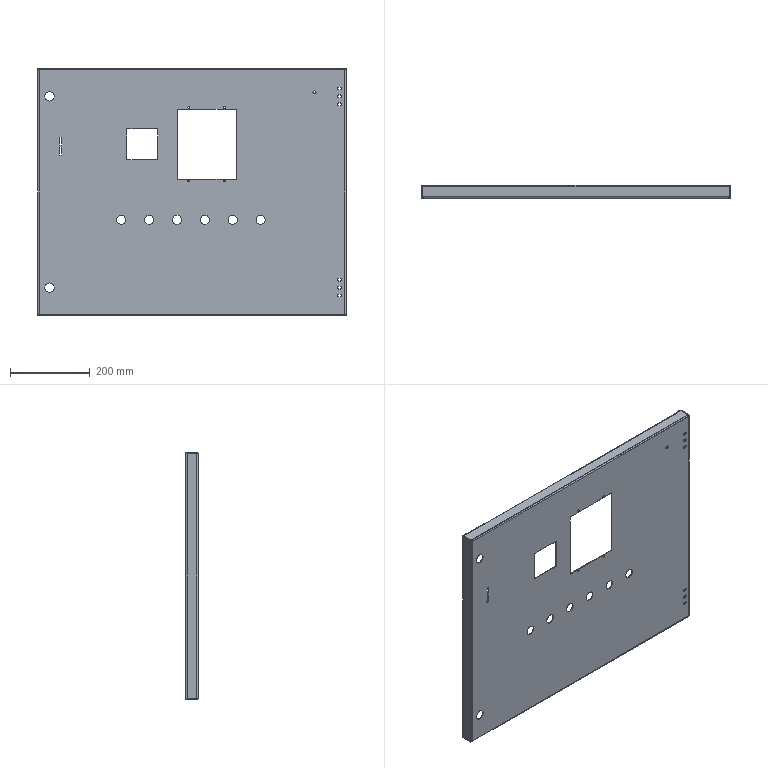Part | STEP file | 1 solid | 180 faces | box 775 x 32 x 620 mm | volume 1109969 mm3 | plane 122 | cylinder 58 | commonest cylinder face diameters 7 x22 23 x12 3 x10 5.3 x8 23.5 x4 7.77 x2